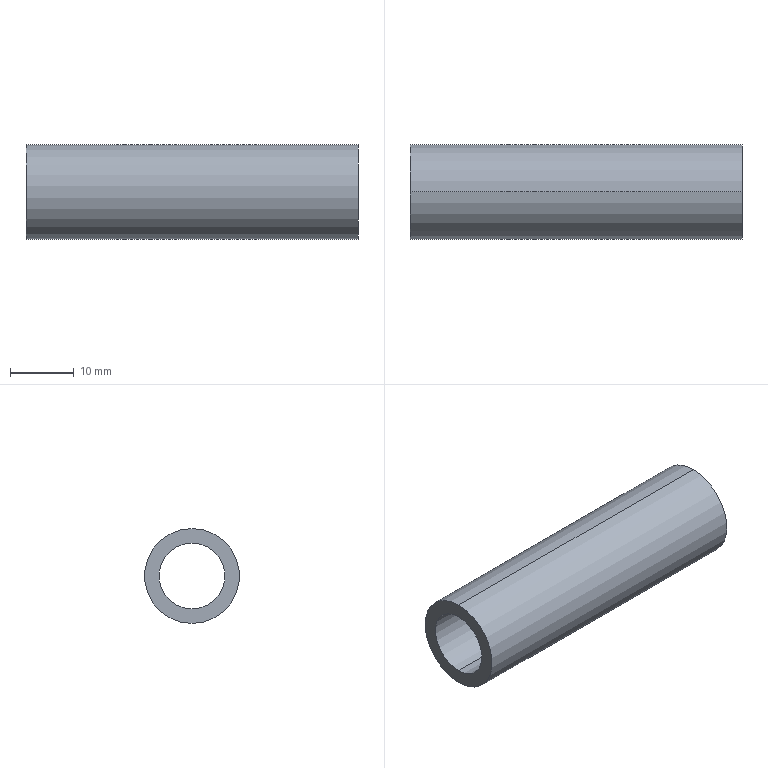Part | NX | features solid 2 | 1 solid | 6 faces | box 52 x 14.85 x 14.85 mm | volume 4674 mm3 | cylinder 4 | plane 2 | commonest cylinder face diameters 10.3 x2 14.85 x2
STEP:
#1=CARTESIAN_POINT('',(216.,-71.5,-169.425));
#2=VERTEX_POINT('',#1);
#3=CARTESIAN_POINT('',(216.,-71.5,-154.575));
#4=VERTEX_POINT('',#3);
#5=CARTESIAN_POINT('',(216.,-71.5,-162.));
#6=DIRECTION('',(-1.,0.,0.));
#7=DIRECTION('',(0.,0.,-1.));
#8=AXIS2_PLACEMENT_3D('',#5,#6,#7);
#9=CIRCLE('',#8,7.425);
#10=EDGE_CURVE('',#2,#4,#9,.T.);
#11=ORIENTED_EDGE('',*,*,#10,.T.);
#12=CARTESIAN_POINT('',(164.,-71.5,-154.575));
#13=VERTEX_POINT('',#12);
#14=CARTESIAN_POINT('',(164.,-71.5,-154.575));
#15=DIRECTION('',(1.,0.,0.));
#16=VECTOR('',#15,1000.);
#17=LINE('',#14,#16);
#18=EDGE_CURVE('',#13,#4,#17,.T.);
#19=ORIENTED_EDGE('',*,*,#18,.F.);
#20=CARTESIAN_POINT('',(164.,-71.5,-169.425));
#21=VERTEX_POINT('',#20);
#22=CARTESIAN_POINT('',(164.,-71.5,-162.));
#23=DIRECTION('',(1.,0.,0.));
#24=DIRECTION('',(0.,0.,1.));
#25=AXIS2_PLACEMENT_3D('',#22,#23,#24);
#26=CIRCLE('',#25,7.425);
#27=EDGE_CURVE('',#13,#21,#26,.T.);
#28=ORIENTED_EDGE('',*,*,#27,.T.);
#29=CARTESIAN_POINT('',(164.,-71.5,-169.425));
#30=DIRECTION('',(1.,0.,0.));
#31=VECTOR('',#30,1000.);
#32=LINE('',#29,#31);
#33=EDGE_CURVE('',#2,#21,#32,.F.);
#34=ORIENTED_EDGE('',*,*,#33,.F.);
#35=EDGE_LOOP('',(#11,#19,#28,#34));
#36=FACE_BOUND('',#35,.T.);
#37=CARTESIAN_POINT('',(216.,-71.5,-162.));
#38=DIRECTION('',(-1.,0.,0.));
#39=DIRECTION('',(0.,0.,-1.));
#40=AXIS2_PLACEMENT_3D('',#37,#38,#39);
#41=CYLINDRICAL_SURFACE('',#40,7.425);
#42=ADVANCED_FACE('',(#36),#41,.T.);
#43=ORIENTED_EDGE('',*,*,#33,.T.);
#44=CARTESIAN_POINT('',(164.,-71.5,-162.));
#45=DIRECTION('',(1.,0.,0.));
#46=DIRECTION('',(0.,0.,-1.));
#47=AXIS2_PLACEMENT_3D('',#44,#45,#46);
#48=CIRCLE('',#47,7.425);
#49=EDGE_CURVE('',#21,#13,#48,.T.);
#50=ORIENTED_EDGE('',*,*,#49,.T.);
#51=ORIENTED_EDGE('',*,*,#18,.T.);
#52=CARTESIAN_POINT('',(216.,-71.5,-162.));
#53=DIRECTION('',(-1.,0.,0.));
#54=DIRECTION('',(0.,0.,1.));
#55=AXIS2_PLACEMENT_3D('',#52,#53,#54);
#56=CIRCLE('',#55,7.425);
#57=EDGE_CURVE('',#4,#2,#56,.T.);
#58=ORIENTED_EDGE('',*,*,#57,.T.);
#59=EDGE_LOOP('',(#43,#50,#51,#58));
#60=FACE_BOUND('',#59,.T.);
#61=CARTESIAN_POINT('',(216.,-71.5,-162.));
#62=DIRECTION('',(-1.,0.,0.));
#63=DIRECTION('',(0.,0.,-1.));
#64=AXIS2_PLACEMENT_3D('',#61,#62,#63);
#65=CYLINDRICAL_SURFACE('',#64,7.425);
#66=ADVANCED_FACE('',(#60),#65,.T.);
#67=ORIENTED_EDGE('',*,*,#10,.F.);
#68=ORIENTED_EDGE('',*,*,#57,.F.);
#69=EDGE_LOOP('',(#67,#68));
#70=FACE_BOUND('',#69,.T.);
#71=CARTESIAN_POINT('',(216.,-71.5,-167.15));
#72=VERTEX_POINT('',#71);
#73=CARTESIAN_POINT('',(216.,-71.5,-156.85));
#74=VERTEX_POINT('',#73);
#75=CARTESIAN_POINT('',(216.,-71.5,-162.));
#76=DIRECTION('',(1.,0.,0.));
#77=DIRECTION('',(0.,0.,-1.));
#78=AXIS2_PLACEMENT_3D('',#75,#76,#77);
#79=CIRCLE('',#78,5.15);
#80=EDGE_CURVE('',#72,#74,#79,.T.);
#81=ORIENTED_EDGE('',*,*,#80,.F.);
#82=CARTESIAN_POINT('',(216.,-71.5,-162.));
#83=DIRECTION('',(1.,0.,0.));
#84=DIRECTION('',(0.,0.,1.));
#85=AXIS2_PLACEMENT_3D('',#82,#83,#84);
#86=CIRCLE('',#85,5.15);
#87=EDGE_CURVE('',#74,#72,#86,.T.);
#88=ORIENTED_EDGE('',*,*,#87,.F.);
#89=EDGE_LOOP('',(#81,#88));
#90=FACE_BOUND('',#89,.T.);
#91=CARTESIAN_POINT('',(216.,-71.5,-162.));
#92=DIRECTION('',(-1.,0.,0.));
#93=DIRECTION('',(0.,0.,-1.));
#94=AXIS2_PLACEMENT_3D('',#91,#92,#93);
#95=PLANE('',#94);
#96=ADVANCED_FACE('',(#70,#90),#95,.F.);
#97=CARTESIAN_POINT('',(164.,-71.5,-167.15));
#98=VERTEX_POINT('',#97);
#99=CARTESIAN_POINT('',(164.,-71.5,-167.15));
#100=DIRECTION('',(1.,0.,0.));
#101=VECTOR('',#100,1000.);
#102=LINE('',#99,#101);
#103=EDGE_CURVE('',#98,#72,#102,.T.);
#104=ORIENTED_EDGE('',*,*,#103,.F.);
#105=CARTESIAN_POINT('',(164.,-71.5,-156.85));
#106=VERTEX_POINT('',#105);
#107=CARTESIAN_POINT('',(164.,-71.5,-162.));
#108=DIRECTION('',(-1.,0.,0.));
#109=DIRECTION('',(0.,0.,-1.));
#110=AXIS2_PLACEMENT_3D('',#107,#108,#109);
#111=CIRCLE('',#110,5.15);
#112=EDGE_CURVE('',#98,#106,#111,.T.);
#113=ORIENTED_EDGE('',*,*,#112,.T.);
#114=CARTESIAN_POINT('',(164.,-71.5,-156.85));
#115=DIRECTION('',(1.,0.,0.));
#116=VECTOR('',#115,1000.);
#117=LINE('',#114,#116);
#118=EDGE_CURVE('',#74,#106,#117,.F.);
#119=ORIENTED_EDGE('',*,*,#118,.F.);
#120=ORIENTED_EDGE('',*,*,#87,.T.);
#121=EDGE_LOOP('',(#104,#113,#119,#120));
#122=FACE_BOUND('',#121,.T.);
#123=CARTESIAN_POINT('',(216.,-71.5,-162.));
#124=DIRECTION('',(-1.,0.,0.));
#125=DIRECTION('',(0.,0.,-1.));
#126=AXIS2_PLACEMENT_3D('',#123,#124,#125);
#127=CYLINDRICAL_SURFACE('',#126,5.15);
#128=ADVANCED_FACE('',(#122),#127,.F.);
#129=ORIENTED_EDGE('',*,*,#80,.T.);
#130=ORIENTED_EDGE('',*,*,#118,.T.);
#131=CARTESIAN_POINT('',(164.,-71.5,-162.));
#132=DIRECTION('',(-1.,0.,0.));
#133=DIRECTION('',(0.,0.,1.));
#134=AXIS2_PLACEMENT_3D('',#131,#132,#133);
#135=CIRCLE('',#134,5.15);
#136=EDGE_CURVE('',#106,#98,#135,.T.);
#137=ORIENTED_EDGE('',*,*,#136,.T.);
#138=ORIENTED_EDGE('',*,*,#103,.T.);
#139=EDGE_LOOP('',(#129,#130,#137,#138));
#140=FACE_BOUND('',#139,.T.);
#141=CARTESIAN_POINT('',(216.,-71.5,-162.));
#142=DIRECTION('',(-1.,0.,0.));
#143=DIRECTION('',(0.,0.,-1.));
#144=AXIS2_PLACEMENT_3D('',#141,#142,#143);
#145=CYLINDRICAL_SURFACE('',#144,5.15);
#146=ADVANCED_FACE('',(#140),#145,.F.);
#147=ORIENTED_EDGE('',*,*,#49,.F.);
#148=ORIENTED_EDGE('',*,*,#27,.F.);
#149=EDGE_LOOP('',(#147,#148));
#150=FACE_BOUND('',#149,.T.);
#151=ORIENTED_EDGE('',*,*,#136,.F.);
#152=ORIENTED_EDGE('',*,*,#112,.F.);
#153=EDGE_LOOP('',(#151,#152));
#154=FACE_BOUND('',#153,.T.);
#155=CARTESIAN_POINT('',(164.,-71.5,-162.));
#156=DIRECTION('',(-1.,0.,0.));
#157=DIRECTION('',(0.,0.,-1.));
#158=AXIS2_PLACEMENT_3D('',#155,#156,#157);
#159=PLANE('',#158);
#160=ADVANCED_FACE('',(#150,#154),#159,.T.);
#161=CLOSED_SHELL('',(#42,#66,#96,#128,#146,#160));
#162=MANIFOLD_SOLID_BREP('',#161);
#163=(LENGTH_UNIT()NAMED_UNIT(*)SI_UNIT(.MILLI.,.METRE.));
#164=UNCERTAINTY_MEASURE_WITH_UNIT(LENGTH_MEASURE(0.00001),#163,'','');
#165=(NAMED_UNIT(*)PLANE_ANGLE_UNIT()SI_UNIT($,.RADIAN.));
#166=(NAMED_UNIT(*)SI_UNIT($,.STERADIAN.)SOLID_ANGLE_UNIT());
#167=(GEOMETRIC_REPRESENTATION_CONTEXT(3)GLOBAL_UNCERTAINTY_ASSIGNED_CONTEXT((#164))GLOBAL_UNIT_ASSIGNED_CONTEXT((#163,#165,#166))REPRESENTATION_CONTEXT('',''));
#168=ADVANCED_BREP_SHAPE_REPRESENTATION('',(#162),#167);